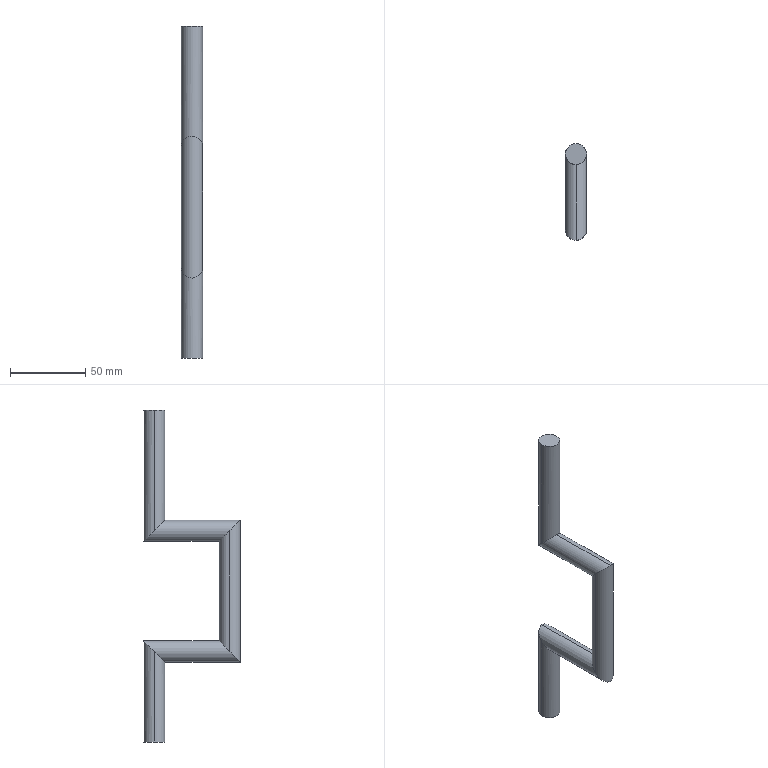Part | SolidWorks | features Sweep 1 | 1 solid | 12 faces | box 14 x 64 x 220 mm | volume 49260 mm3 | cylinder 10 | plane 2 | commonest cylinder face diameters 14 x10
STEP:
#1=CARTESIAN_POINT('',(7.,0.,0.));
#2=VERTEX_POINT('',#1);
#3=CARTESIAN_POINT('',(-7.,0.,0.));
#4=VERTEX_POINT('',#3);
#5=CARTESIAN_POINT('',(0.,0.,0.));
#6=DIRECTION('',(0.,0.,1.));
#7=DIRECTION('',(1.,0.,0.));
#8=AXIS2_PLACEMENT_3D('',#5,#6,#7);
#9=CIRCLE('',#8,7.);
#10=EDGE_CURVE('',#2,#4,#9,.T.);
#11=ORIENTED_EDGE('',*,*,#10,.F.);
#12=CARTESIAN_POINT('',(7.,0.,-80.));
#13=VERTEX_POINT('',#12);
#14=CARTESIAN_POINT('',(7.,0.,0.));
#15=DIRECTION('',(0.,0.,-1.));
#16=VECTOR('',#15,1000.);
#17=LINE('',#14,#16);
#18=EDGE_CURVE('',#2,#13,#17,.T.);
#19=ORIENTED_EDGE('',*,*,#18,.T.);
#20=CARTESIAN_POINT('',(0.,7.,-87.));
#21=VERTEX_POINT('',#20);
#22=CARTESIAN_POINT('',(0.,7.,-87.));
#23=CARTESIAN_POINT('',(4.101,7.,-87.));
#24=CARTESIAN_POINT('',(7.,4.101,-84.101));
#25=CARTESIAN_POINT('',(7.,0.,-80.));
#26=(BOUNDED_CURVE()B_SPLINE_CURVE(3,(#22,#23,#24,#25),.UNSPECIFIED.,.F.,.F.)B_SPLINE_CURVE_WITH_KNOTS((4,4),(0.,1.571),.UNSPECIFIED.)CURVE()GEOMETRIC_REPRESENTATION_ITEM()RATIONAL_B_SPLINE_CURVE((1.,0.8047,0.8047,1.))REPRESENTATION_ITEM(''));
#27=EDGE_CURVE('',#21,#13,#26,.T.);
#28=ORIENTED_EDGE('',*,*,#27,.F.);
#29=CARTESIAN_POINT('',(-7.,0.,-80.));
#30=VERTEX_POINT('',#29);
#31=CARTESIAN_POINT('',(-7.,0.,-80.));
#32=CARTESIAN_POINT('',(-7.,4.101,-84.101));
#33=CARTESIAN_POINT('',(-4.101,7.,-87.));
#34=CARTESIAN_POINT('',(0.,7.,-87.));
#35=(BOUNDED_CURVE()B_SPLINE_CURVE(3,(#31,#32,#33,#34),.UNSPECIFIED.,.F.,.F.)B_SPLINE_CURVE_WITH_KNOTS((4,4),(4.712,6.283),.UNSPECIFIED.)CURVE()GEOMETRIC_REPRESENTATION_ITEM()RATIONAL_B_SPLINE_CURVE((1.,0.8047,0.8047,1.))REPRESENTATION_ITEM(''));
#36=EDGE_CURVE('',#30,#21,#35,.T.);
#37=ORIENTED_EDGE('',*,*,#36,.F.);
#38=CARTESIAN_POINT('',(-7.,0.,0.));
#39=DIRECTION('',(0.,0.,-1.));
#40=VECTOR('',#39,1000.);
#41=LINE('',#38,#40);
#42=EDGE_CURVE('',#4,#30,#41,.T.);
#43=ORIENTED_EDGE('',*,*,#42,.F.);
#44=EDGE_LOOP('',(#11,#19,#28,#37,#43));
#45=FACE_OUTER_BOUND('',#44,.T.);
#46=CARTESIAN_POINT('',(0.,0.,0.));
#47=DIRECTION('',(0.,0.,-1.));
#48=DIRECTION('',(-1.,0.,0.));
#49=AXIS2_PLACEMENT_3D('',#46,#47,#48);
#50=CYLINDRICAL_SURFACE('',#49,7.);
#51=ADVANCED_FACE('',(#45),#50,.T.);
#52=ORIENTED_EDGE('',*,*,#27,.T.);
#53=CARTESIAN_POINT('',(0.,-7.,-73.));
#54=VERTEX_POINT('',#53);
#55=CARTESIAN_POINT('',(7.,0.,-80.));
#56=CARTESIAN_POINT('',(7.,-4.101,-75.899));
#57=CARTESIAN_POINT('',(4.101,-7.,-73.));
#58=CARTESIAN_POINT('',(0.,-7.,-73.));
#59=(BOUNDED_CURVE()B_SPLINE_CURVE(3,(#55,#56,#57,#58),.UNSPECIFIED.,.F.,.T.)B_SPLINE_CURVE_WITH_KNOTS((4,4),(1.571,3.142),.UNSPECIFIED.)CURVE()GEOMETRIC_REPRESENTATION_ITEM()RATIONAL_B_SPLINE_CURVE((1.,0.8047,0.8047,1.))REPRESENTATION_ITEM(''));
#60=EDGE_CURVE('',#13,#54,#59,.T.);
#61=ORIENTED_EDGE('',*,*,#60,.T.);
#62=CARTESIAN_POINT('',(0.,-57.,-73.));
#63=VERTEX_POINT('',#62);
#64=CARTESIAN_POINT('',(0.,15.5,-73.));
#65=DIRECTION('',(0.,-1.,0.));
#66=VECTOR('',#65,1000.);
#67=LINE('',#64,#66);
#68=EDGE_CURVE('',#54,#63,#67,.T.);
#69=ORIENTED_EDGE('',*,*,#68,.T.);
#70=CARTESIAN_POINT('',(7.,-50.,-80.));
#71=VERTEX_POINT('',#70);
#72=CARTESIAN_POINT('',(7.,-50.,-80.));
#73=CARTESIAN_POINT('',(7.,-54.101,-75.899));
#74=CARTESIAN_POINT('',(4.101,-57.,-73.));
#75=CARTESIAN_POINT('',(0.,-57.,-73.));
#76=(BOUNDED_CURVE()B_SPLINE_CURVE(3,(#72,#73,#74,#75),.UNSPECIFIED.,.F.,.F.)B_SPLINE_CURVE_WITH_KNOTS((4,4),(4.712,6.283),.UNSPECIFIED.)CURVE()GEOMETRIC_REPRESENTATION_ITEM()RATIONAL_B_SPLINE_CURVE((1.,0.8047,0.8047,1.))REPRESENTATION_ITEM(''));
#77=EDGE_CURVE('',#71,#63,#76,.T.);
#78=ORIENTED_EDGE('',*,*,#77,.F.);
#79=CARTESIAN_POINT('',(0.,-43.,-87.));
#80=VERTEX_POINT('',#79);
#81=CARTESIAN_POINT('',(0.,-43.,-87.));
#82=CARTESIAN_POINT('',(4.101,-43.,-87.));
#83=CARTESIAN_POINT('',(7.,-45.899,-84.101));
#84=CARTESIAN_POINT('',(7.,-50.,-80.));
#85=(BOUNDED_CURVE()B_SPLINE_CURVE(3,(#81,#82,#83,#84),.UNSPECIFIED.,.F.,.F.)B_SPLINE_CURVE_WITH_KNOTS((4,4),(3.142,4.712),.UNSPECIFIED.)CURVE()GEOMETRIC_REPRESENTATION_ITEM()RATIONAL_B_SPLINE_CURVE((1.,0.8047,0.8047,1.))REPRESENTATION_ITEM(''));
#86=EDGE_CURVE('',#80,#71,#85,.T.);
#87=ORIENTED_EDGE('',*,*,#86,.F.);
#88=CARTESIAN_POINT('',(0.,15.5,-87.));
#89=DIRECTION('',(0.,-1.,0.));
#90=VECTOR('',#89,1000.);
#91=LINE('',#88,#90);
#92=EDGE_CURVE('',#21,#80,#91,.T.);
#93=ORIENTED_EDGE('',*,*,#92,.F.);
#94=EDGE_LOOP('',(#52,#61,#69,#78,#87,#93));
#95=FACE_OUTER_BOUND('',#94,.T.);
#96=CARTESIAN_POINT('',(0.,15.5,-80.));
#97=DIRECTION('',(0.,-1.,0.));
#98=DIRECTION('',(0.,0.,-1.));
#99=AXIS2_PLACEMENT_3D('',#96,#97,#98);
#100=CYLINDRICAL_SURFACE('',#99,7.);
#101=ADVANCED_FACE('',(#95),#100,.T.);
#102=CARTESIAN_POINT('',(-7.,-50.,-80.));
#103=VERTEX_POINT('',#102);
#104=CARTESIAN_POINT('',(-7.,-50.,-80.));
#105=CARTESIAN_POINT('',(-7.,-45.899,-84.101));
#106=CARTESIAN_POINT('',(-4.101,-43.,-87.));
#107=CARTESIAN_POINT('',(0.,-43.,-87.));
#108=(BOUNDED_CURVE()B_SPLINE_CURVE(3,(#104,#105,#106,#107),.UNSPECIFIED.,.F.,.F.)B_SPLINE_CURVE_WITH_KNOTS((4,4),(1.571,3.142),.UNSPECIFIED.)CURVE()GEOMETRIC_REPRESENTATION_ITEM()RATIONAL_B_SPLINE_CURVE((1.,0.8047,0.8047,1.))REPRESENTATION_ITEM(''));
#109=EDGE_CURVE('',#103,#80,#108,.T.);
#110=ORIENTED_EDGE('',*,*,#109,.T.);
#111=ORIENTED_EDGE('',*,*,#86,.T.);
#112=CARTESIAN_POINT('',(7.,-50.,-160.));
#113=VERTEX_POINT('',#112);
#114=CARTESIAN_POINT('',(7.,-50.,-64.5));
#115=DIRECTION('',(0.,0.,-1.));
#116=VECTOR('',#115,1000.);
#117=LINE('',#114,#116);
#118=EDGE_CURVE('',#71,#113,#117,.T.);
#119=ORIENTED_EDGE('',*,*,#118,.T.);
#120=CARTESIAN_POINT('',(0.,-43.,-153.));
#121=VERTEX_POINT('',#120);
#122=CARTESIAN_POINT('',(0.,-43.,-153.));
#123=CARTESIAN_POINT('',(4.101,-43.,-153.));
#124=CARTESIAN_POINT('',(7.,-45.899,-155.899));
#125=CARTESIAN_POINT('',(7.,-50.,-160.));
#126=(BOUNDED_CURVE()B_SPLINE_CURVE(3,(#122,#123,#124,#125),.UNSPECIFIED.,.F.,.F.)B_SPLINE_CURVE_WITH_KNOTS((4,4),(3.142,4.712),.UNSPECIFIED.)CURVE()GEOMETRIC_REPRESENTATION_ITEM()RATIONAL_B_SPLINE_CURVE((1.,0.8047,0.8047,1.))REPRESENTATION_ITEM(''));
#127=EDGE_CURVE('',#121,#113,#126,.T.);
#128=ORIENTED_EDGE('',*,*,#127,.F.);
#129=CARTESIAN_POINT('',(-7.,-50.,-160.));
#130=VERTEX_POINT('',#129);
#131=CARTESIAN_POINT('',(-7.,-50.,-160.));
#132=CARTESIAN_POINT('',(-7.,-45.899,-155.899));
#133=CARTESIAN_POINT('',(-4.101,-43.,-153.));
#134=CARTESIAN_POINT('',(0.,-43.,-153.));
#135=(BOUNDED_CURVE()B_SPLINE_CURVE(3,(#131,#132,#133,#134),.UNSPECIFIED.,.F.,.F.)B_SPLINE_CURVE_WITH_KNOTS((4,4),(1.571,3.142),.UNSPECIFIED.)CURVE()GEOMETRIC_REPRESENTATION_ITEM()RATIONAL_B_SPLINE_CURVE((1.,0.8047,0.8047,1.))REPRESENTATION_ITEM(''));
#136=EDGE_CURVE('',#130,#121,#135,.T.);
#137=ORIENTED_EDGE('',*,*,#136,.F.);
#138=CARTESIAN_POINT('',(-7.,-50.,-64.5));
#139=DIRECTION('',(0.,0.,-1.));
#140=VECTOR('',#139,1000.);
#141=LINE('',#138,#140);
#142=EDGE_CURVE('',#103,#130,#141,.T.);
#143=ORIENTED_EDGE('',*,*,#142,.F.);
#144=EDGE_LOOP('',(#110,#111,#119,#128,#137,#143));
#145=FACE_OUTER_BOUND('',#144,.T.);
#146=CARTESIAN_POINT('',(0.,-50.,-64.5));
#147=DIRECTION('',(0.,0.,-1.));
#148=DIRECTION('',(-1.,0.,0.));
#149=AXIS2_PLACEMENT_3D('',#146,#147,#148);
#150=CYLINDRICAL_SURFACE('',#149,7.);
#151=ADVANCED_FACE('',(#145),#150,.T.);
#152=ORIENTED_EDGE('',*,*,#127,.T.);
#153=CARTESIAN_POINT('',(0.,-57.,-167.));
#154=VERTEX_POINT('',#153);
#155=CARTESIAN_POINT('',(7.,-50.,-160.));
#156=CARTESIAN_POINT('',(7.,-54.101,-164.101));
#157=CARTESIAN_POINT('',(4.101,-57.,-167.));
#158=CARTESIAN_POINT('',(0.,-57.,-167.));
#159=(BOUNDED_CURVE()B_SPLINE_CURVE(3,(#155,#156,#157,#158),.UNSPECIFIED.,.F.,.F.)B_SPLINE_CURVE_WITH_KNOTS((4,4),(4.712,6.283),.UNSPECIFIED.)CURVE()GEOMETRIC_REPRESENTATION_ITEM()RATIONAL_B_SPLINE_CURVE((1.,0.8047,0.8047,1.))REPRESENTATION_ITEM(''));
#160=EDGE_CURVE('',#113,#154,#159,.T.);
#161=ORIENTED_EDGE('',*,*,#160,.T.);
#162=CARTESIAN_POINT('',(0.,-7.,-167.));
#163=VERTEX_POINT('',#162);
#164=CARTESIAN_POINT('',(0.,-65.5,-167.));
#165=DIRECTION('',(0.,1.,0.));
#166=VECTOR('',#165,1000.);
#167=LINE('',#164,#166);
#168=EDGE_CURVE('',#154,#163,#167,.T.);
#169=ORIENTED_EDGE('',*,*,#168,.T.);
#170=CARTESIAN_POINT('',(7.,0.,-160.));
#171=VERTEX_POINT('',#170);
#172=CARTESIAN_POINT('',(7.,0.,-160.));
#173=CARTESIAN_POINT('',(7.,-4.101,-164.101));
#174=CARTESIAN_POINT('',(4.101,-7.,-167.));
#175=CARTESIAN_POINT('',(0.,-7.,-167.));
#176=(BOUNDED_CURVE()B_SPLINE_CURVE(3,(#172,#173,#174,#175),.UNSPECIFIED.,.F.,.F.)B_SPLINE_CURVE_WITH_KNOTS((4,4),(1.571,3.142),.UNSPECIFIED.)CURVE()GEOMETRIC_REPRESENTATION_ITEM()RATIONAL_B_SPLINE_CURVE((1.,0.8047,0.8047,1.))REPRESENTATION_ITEM(''));
#177=EDGE_CURVE('',#171,#163,#176,.T.);
#178=ORIENTED_EDGE('',*,*,#177,.F.);
#179=CARTESIAN_POINT('',(0.,7.,-153.));
#180=VERTEX_POINT('',#179);
#181=CARTESIAN_POINT('',(0.,7.,-153.));
#182=CARTESIAN_POINT('',(4.101,7.,-153.));
#183=CARTESIAN_POINT('',(7.,4.101,-155.899));
#184=CARTESIAN_POINT('',(7.,0.,-160.));
#185=(BOUNDED_CURVE()B_SPLINE_CURVE(3,(#181,#182,#183,#184),.UNSPECIFIED.,.F.,.F.)B_SPLINE_CURVE_WITH_KNOTS((4,4),(0.,1.571),.UNSPECIFIED.)CURVE()GEOMETRIC_REPRESENTATION_ITEM()RATIONAL_B_SPLINE_CURVE((1.,0.8047,0.8047,1.))REPRESENTATION_ITEM(''));
#186=EDGE_CURVE('',#180,#171,#185,.T.);
#187=ORIENTED_EDGE('',*,*,#186,.F.);
#188=CARTESIAN_POINT('',(0.,-65.5,-153.));
#189=DIRECTION('',(0.,1.,0.));
#190=VECTOR('',#189,1000.);
#191=LINE('',#188,#190);
#192=EDGE_CURVE('',#121,#180,#191,.T.);
#193=ORIENTED_EDGE('',*,*,#192,.F.);
#194=EDGE_LOOP('',(#152,#161,#169,#178,#187,#193));
#195=FACE_OUTER_BOUND('',#194,.T.);
#196=CARTESIAN_POINT('',(0.,-65.5,-160.));
#197=DIRECTION('',(0.,1.,0.));
#198=DIRECTION('',(0.,0.,1.));
#199=AXIS2_PLACEMENT_3D('',#196,#197,#198);
#200=CYLINDRICAL_SURFACE('',#199,7.);
#201=ADVANCED_FACE('',(#195),#200,.T.);
#202=CARTESIAN_POINT('',(-7.,0.,-160.));
#203=VERTEX_POINT('',#202);
#204=CARTESIAN_POINT('',(-7.,0.,-160.));
#205=CARTESIAN_POINT('',(-7.,4.101,-155.899));
#206=CARTESIAN_POINT('',(-4.101,7.,-153.));
#207=CARTESIAN_POINT('',(0.,7.,-153.));
#208=(BOUNDED_CURVE()B_SPLINE_CURVE(3,(#204,#205,#206,#207),.UNSPECIFIED.,.F.,.T.)B_SPLINE_CURVE_WITH_KNOTS((4,4),(4.712,6.283),.UNSPECIFIED.)CURVE()GEOMETRIC_REPRESENTATION_ITEM()RATIONAL_B_SPLINE_CURVE((1.,0.8047,0.8047,1.))REPRESENTATION_ITEM(''));
#209=EDGE_CURVE('',#203,#180,#208,.T.);
#210=ORIENTED_EDGE('',*,*,#209,.T.);
#211=ORIENTED_EDGE('',*,*,#186,.T.);
#212=CARTESIAN_POINT('',(7.,0.,-220.));
#213=VERTEX_POINT('',#212);
#214=CARTESIAN_POINT('',(7.,0.,-144.5));
#215=DIRECTION('',(0.,0.,-1.));
#216=VECTOR('',#215,1000.);
#217=LINE('',#214,#216);
#218=EDGE_CURVE('',#171,#213,#217,.T.);
#219=ORIENTED_EDGE('',*,*,#218,.T.);
#220=CARTESIAN_POINT('',(-7.,0.,-220.));
#221=VERTEX_POINT('',#220);
#222=CARTESIAN_POINT('',(0.,0.,-220.));
#223=DIRECTION('',(0.,0.,1.));
#224=DIRECTION('',(1.,0.,0.));
#225=AXIS2_PLACEMENT_3D('',#222,#223,#224);
#226=CIRCLE('',#225,7.);
#227=EDGE_CURVE('',#213,#221,#226,.T.);
#228=ORIENTED_EDGE('',*,*,#227,.T.);
#229=CARTESIAN_POINT('',(-7.,0.,-144.5));
#230=DIRECTION('',(0.,0.,-1.));
#231=VECTOR('',#230,1000.);
#232=LINE('',#229,#231);
#233=EDGE_CURVE('',#203,#221,#232,.T.);
#234=ORIENTED_EDGE('',*,*,#233,.F.);
#235=EDGE_LOOP('',(#210,#211,#219,#228,#234));
#236=FACE_OUTER_BOUND('',#235,.T.);
#237=CARTESIAN_POINT('',(0.,0.,-144.5));
#238=DIRECTION('',(0.,0.,-1.));
#239=DIRECTION('',(-1.,0.,0.));
#240=AXIS2_PLACEMENT_3D('',#237,#238,#239);
#241=CYLINDRICAL_SURFACE('',#240,7.);
#242=ADVANCED_FACE('',(#236),#241,.T.);
#243=ORIENTED_EDGE('',*,*,#18,.F.);
#244=CARTESIAN_POINT('',(0.,0.,0.));
#245=DIRECTION('',(0.,0.,1.));
#246=DIRECTION('',(1.,0.,0.));
#247=AXIS2_PLACEMENT_3D('',#244,#245,#246);
#248=CIRCLE('',#247,7.);
#249=EDGE_CURVE('',#4,#2,#248,.T.);
#250=ORIENTED_EDGE('',*,*,#249,.F.);
#251=ORIENTED_EDGE('',*,*,#42,.T.);
#252=CARTESIAN_POINT('',(0.,-7.,-73.));
#253=CARTESIAN_POINT('',(-4.101,-7.,-73.));
#254=CARTESIAN_POINT('',(-7.,-4.101,-75.899));
#255=CARTESIAN_POINT('',(-7.,0.,-80.));
#256=(BOUNDED_CURVE()B_SPLINE_CURVE(3,(#252,#253,#254,#255),.UNSPECIFIED.,.F.,.T.)B_SPLINE_CURVE_WITH_KNOTS((4,4),(3.142,4.712),.UNSPECIFIED.)CURVE()GEOMETRIC_REPRESENTATION_ITEM()RATIONAL_B_SPLINE_CURVE((1.,0.8047,0.8047,1.))REPRESENTATION_ITEM(''));
#257=EDGE_CURVE('',#54,#30,#256,.T.);
#258=ORIENTED_EDGE('',*,*,#257,.F.);
#259=ORIENTED_EDGE('',*,*,#60,.F.);
#260=EDGE_LOOP('',(#243,#250,#251,#258,#259));
#261=FACE_OUTER_BOUND('',#260,.T.);
#262=CARTESIAN_POINT('',(0.,0.,0.));
#263=DIRECTION('',(0.,0.,-1.));
#264=DIRECTION('',(-1.,0.,0.));
#265=AXIS2_PLACEMENT_3D('',#262,#263,#264);
#266=CYLINDRICAL_SURFACE('',#265,7.);
#267=ADVANCED_FACE('',(#261),#266,.T.);
#268=ORIENTED_EDGE('',*,*,#68,.F.);
#269=ORIENTED_EDGE('',*,*,#257,.T.);
#270=ORIENTED_EDGE('',*,*,#36,.T.);
#271=ORIENTED_EDGE('',*,*,#92,.T.);
#272=ORIENTED_EDGE('',*,*,#109,.F.);
#273=CARTESIAN_POINT('',(0.,-57.,-73.));
#274=CARTESIAN_POINT('',(-4.101,-57.,-73.));
#275=CARTESIAN_POINT('',(-7.,-54.101,-75.899));
#276=CARTESIAN_POINT('',(-7.,-50.,-80.));
#277=(BOUNDED_CURVE()B_SPLINE_CURVE(3,(#273,#274,#275,#276),.UNSPECIFIED.,.F.,.F.)B_SPLINE_CURVE_WITH_KNOTS((4,4),(0.,1.571),.UNSPECIFIED.)CURVE()GEOMETRIC_REPRESENTATION_ITEM()RATIONAL_B_SPLINE_CURVE((1.,0.8047,0.8047,1.))REPRESENTATION_ITEM(''));
#278=EDGE_CURVE('',#63,#103,#277,.T.);
#279=ORIENTED_EDGE('',*,*,#278,.F.);
#280=EDGE_LOOP('',(#268,#269,#270,#271,#272,#279));
#281=FACE_OUTER_BOUND('',#280,.T.);
#282=CARTESIAN_POINT('',(0.,15.5,-80.));
#283=DIRECTION('',(0.,-1.,0.));
#284=DIRECTION('',(0.,0.,-1.));
#285=AXIS2_PLACEMENT_3D('',#282,#283,#284);
#286=CYLINDRICAL_SURFACE('',#285,7.);
#287=ADVANCED_FACE('',(#281),#286,.T.);
#288=ORIENTED_EDGE('',*,*,#118,.F.);
#289=ORIENTED_EDGE('',*,*,#77,.T.);
#290=ORIENTED_EDGE('',*,*,#278,.T.);
#291=ORIENTED_EDGE('',*,*,#142,.T.);
#292=CARTESIAN_POINT('',(0.,-57.,-167.));
#293=CARTESIAN_POINT('',(-4.101,-57.,-167.));
#294=CARTESIAN_POINT('',(-7.,-54.101,-164.101));
#295=CARTESIAN_POINT('',(-7.,-50.,-160.));
#296=(BOUNDED_CURVE()B_SPLINE_CURVE(3,(#292,#293,#294,#295),.UNSPECIFIED.,.F.,.F.)B_SPLINE_CURVE_WITH_KNOTS((4,4),(0.,1.571),.UNSPECIFIED.)CURVE()GEOMETRIC_REPRESENTATION_ITEM()RATIONAL_B_SPLINE_CURVE((1.,0.8047,0.8047,1.))REPRESENTATION_ITEM(''));
#297=EDGE_CURVE('',#154,#130,#296,.T.);
#298=ORIENTED_EDGE('',*,*,#297,.F.);
#299=ORIENTED_EDGE('',*,*,#160,.F.);
#300=EDGE_LOOP('',(#288,#289,#290,#291,#298,#299));
#301=FACE_OUTER_BOUND('',#300,.T.);
#302=CARTESIAN_POINT('',(0.,-50.,-64.5));
#303=DIRECTION('',(0.,0.,-1.));
#304=DIRECTION('',(-1.,0.,0.));
#305=AXIS2_PLACEMENT_3D('',#302,#303,#304);
#306=CYLINDRICAL_SURFACE('',#305,7.);
#307=ADVANCED_FACE('',(#301),#306,.T.);
#308=ORIENTED_EDGE('',*,*,#168,.F.);
#309=ORIENTED_EDGE('',*,*,#297,.T.);
#310=ORIENTED_EDGE('',*,*,#136,.T.);
#311=ORIENTED_EDGE('',*,*,#192,.T.);
#312=ORIENTED_EDGE('',*,*,#209,.F.);
#313=CARTESIAN_POINT('',(0.,-7.,-167.));
#314=CARTESIAN_POINT('',(-4.101,-7.,-167.));
#315=CARTESIAN_POINT('',(-7.,-4.101,-164.101));
#316=CARTESIAN_POINT('',(-7.,0.,-160.));
#317=(BOUNDED_CURVE()B_SPLINE_CURVE(3,(#313,#314,#315,#316),.UNSPECIFIED.,.F.,.F.)B_SPLINE_CURVE_WITH_KNOTS((4,4),(3.142,4.712),.UNSPECIFIED.)CURVE()GEOMETRIC_REPRESENTATION_ITEM()RATIONAL_B_SPLINE_CURVE((1.,0.8047,0.8047,1.))REPRESENTATION_ITEM(''));
#318=EDGE_CURVE('',#163,#203,#317,.T.);
#319=ORIENTED_EDGE('',*,*,#318,.F.);
#320=EDGE_LOOP('',(#308,#309,#310,#311,#312,#319));
#321=FACE_OUTER_BOUND('',#320,.T.);
#322=CARTESIAN_POINT('',(0.,-65.5,-160.));
#323=DIRECTION('',(0.,1.,0.));
#324=DIRECTION('',(0.,0.,1.));
#325=AXIS2_PLACEMENT_3D('',#322,#323,#324);
#326=CYLINDRICAL_SURFACE('',#325,7.);
#327=ADVANCED_FACE('',(#321),#326,.T.);
#328=ORIENTED_EDGE('',*,*,#218,.F.);
#329=ORIENTED_EDGE('',*,*,#177,.T.);
#330=ORIENTED_EDGE('',*,*,#318,.T.);
#331=ORIENTED_EDGE('',*,*,#233,.T.);
#332=CARTESIAN_POINT('',(0.,0.,-220.));
#333=DIRECTION('',(0.,0.,1.));
#334=DIRECTION('',(1.,0.,0.));
#335=AXIS2_PLACEMENT_3D('',#332,#333,#334);
#336=CIRCLE('',#335,7.);
#337=EDGE_CURVE('',#221,#213,#336,.T.);
#338=ORIENTED_EDGE('',*,*,#337,.T.);
#339=EDGE_LOOP('',(#328,#329,#330,#331,#338));
#340=FACE_OUTER_BOUND('',#339,.T.);
#341=CARTESIAN_POINT('',(0.,0.,-144.5));
#342=DIRECTION('',(0.,0.,-1.));
#343=DIRECTION('',(-1.,0.,0.));
#344=AXIS2_PLACEMENT_3D('',#341,#342,#343);
#345=CYLINDRICAL_SURFACE('',#344,7.);
#346=ADVANCED_FACE('',(#340),#345,.T.);
#347=ORIENTED_EDGE('',*,*,#249,.T.);
#348=ORIENTED_EDGE('',*,*,#10,.T.);
#349=EDGE_LOOP('',(#347,#348));
#350=FACE_OUTER_BOUND('',#349,.T.);
#351=CARTESIAN_POINT('',(0.,0.,0.));
#352=DIRECTION('',(0.,0.,1.));
#353=DIRECTION('',(1.,0.,0.));
#354=AXIS2_PLACEMENT_3D('',#351,#352,#353);
#355=PLANE('',#354);
#356=ADVANCED_FACE('',(#350),#355,.T.);
#357=ORIENTED_EDGE('',*,*,#337,.F.);
#358=ORIENTED_EDGE('',*,*,#227,.F.);
#359=EDGE_LOOP('',(#357,#358));
#360=FACE_OUTER_BOUND('',#359,.T.);
#361=CARTESIAN_POINT('',(0.,0.,-220.));
#362=DIRECTION('',(0.,0.,1.));
#363=DIRECTION('',(1.,0.,0.));
#364=AXIS2_PLACEMENT_3D('',#361,#362,#363);
#365=PLANE('',#364);
#366=ADVANCED_FACE('',(#360),#365,.F.);
#367=CLOSED_SHELL('',(#51,#101,#151,#201,#242,#267,#287,#307,#327,#346,#356,#366));
#368=MANIFOLD_SOLID_BREP('',#367);
#369=CARTESIAN_POINT('',(0.,0.,0.));
#370=DIRECTION('',(0.,0.,1.));
#371=DIRECTION('',(1.,0.,0.));
#372=AXIS2_PLACEMENT_3D('',#369,#370,#371);
#373=(LENGTH_UNIT()NAMED_UNIT(*)SI_UNIT(.MILLI.,.METRE.));
#374=UNCERTAINTY_MEASURE_WITH_UNIT(LENGTH_MEASURE(0.00001),#373,'','');
#375=(NAMED_UNIT(*)PLANE_ANGLE_UNIT()SI_UNIT($,.RADIAN.));
#376=(NAMED_UNIT(*)SI_UNIT($,.STERADIAN.)SOLID_ANGLE_UNIT());
#377=(GEOMETRIC_REPRESENTATION_CONTEXT(3)GLOBAL_UNCERTAINTY_ASSIGNED_CONTEXT((#374))GLOBAL_UNIT_ASSIGNED_CONTEXT((#373,#375,#376))REPRESENTATION_CONTEXT('',''));
#378=ADVANCED_BREP_SHAPE_REPRESENTATION('',(#368,#372),#377);